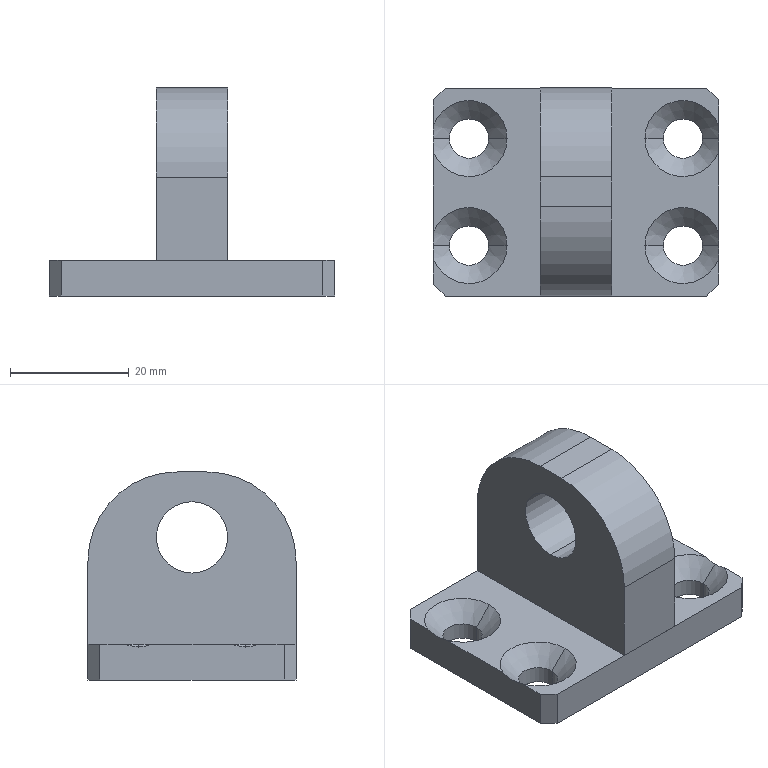Part | SolidWorks | features ICE 2, Chamfer 1, Extrusion 1, Fillet 1, HoleWzd 1 | 2 solids | 36 faces | box 48 x 35 x 35 mm | volume 18352 mm3 | plane 16 | cylinder 12 | cone 8 | commonest cylinder face diameters 6.6 x8 12 x2 30 x2
STEP:
#1=CARTESIAN_POINT('',(-6.,0.,30.));
#2=VERTEX_POINT('',#1);
#3=CARTESIAN_POINT('',(-6.,0.,18.));
#4=VERTEX_POINT('',#3);
#5=CARTESIAN_POINT('',(-6.,0.,24.));
#6=DIRECTION('',(1.,0.,0.));
#7=DIRECTION('',(0.,1.,0.));
#8=AXIS2_PLACEMENT_3D('',#5,#6,#7);
#9=CIRCLE('',#8,6.);
#10=EDGE_CURVE('',#2,#4,#9,.T.);
#11=ORIENTED_EDGE('',*,*,#10,.F.);
#12=CARTESIAN_POINT('',(6.,0.,30.));
#13=VERTEX_POINT('',#12);
#14=CARTESIAN_POINT('',(-14.,0.,30.));
#15=DIRECTION('',(1.,0.,0.));
#16=VECTOR('',#15,1000.);
#17=LINE('',#14,#16);
#18=EDGE_CURVE('',#2,#13,#17,.T.);
#19=ORIENTED_EDGE('',*,*,#18,.T.);
#20=CARTESIAN_POINT('',(6.,0.,18.));
#21=VERTEX_POINT('',#20);
#22=CARTESIAN_POINT('',(6.,0.,24.));
#23=DIRECTION('',(1.,0.,0.));
#24=DIRECTION('',(0.,0.,-1.));
#25=AXIS2_PLACEMENT_3D('',#22,#23,#24);
#26=CIRCLE('',#25,6.);
#27=EDGE_CURVE('',#13,#21,#26,.T.);
#28=ORIENTED_EDGE('',*,*,#27,.T.);
#29=CARTESIAN_POINT('',(-14.,0.,18.));
#30=DIRECTION('',(1.,0.,0.));
#31=VECTOR('',#30,1000.);
#32=LINE('',#29,#31);
#33=EDGE_CURVE('',#4,#21,#32,.T.);
#34=ORIENTED_EDGE('',*,*,#33,.F.);
#35=EDGE_LOOP('',(#11,#19,#28,#34));
#36=FACE_OUTER_BOUND('',#35,.T.);
#37=CARTESIAN_POINT('',(-14.,0.,24.));
#38=DIRECTION('',(1.,0.,0.));
#39=DIRECTION('',(0.,0.,-1.));
#40=AXIS2_PLACEMENT_3D('',#37,#38,#39);
#41=CYLINDRICAL_SURFACE('',#40,6.);
#42=ADVANCED_FACE('',(#36),#41,.F.);
#43=CARTESIAN_POINT('',(6.,0.,24.));
#44=DIRECTION('',(1.,0.,0.));
#45=DIRECTION('',(0.,0.,-1.));
#46=AXIS2_PLACEMENT_3D('',#43,#44,#45);
#47=CIRCLE('',#46,6.);
#48=EDGE_CURVE('',#21,#13,#47,.T.);
#49=ORIENTED_EDGE('',*,*,#48,.F.);
#50=ORIENTED_EDGE('',*,*,#27,.F.);
#51=EDGE_LOOP('',(#49,#50));
#52=FACE_BOUND('',#51,.T.);
#53=CARTESIAN_POINT('',(6.,-2.5,35.));
#54=VERTEX_POINT('',#53);
#55=CARTESIAN_POINT('',(6.,2.5,35.));
#56=VERTEX_POINT('',#55);
#57=CARTESIAN_POINT('',(6.,17.5,35.));
#58=DIRECTION('',(0.,1.,0.));
#59=VECTOR('',#58,1000.);
#60=LINE('',#57,#59);
#61=EDGE_CURVE('',#54,#56,#60,.T.);
#62=ORIENTED_EDGE('',*,*,#61,.F.);
#63=CARTESIAN_POINT('',(6.,-17.5,20.));
#64=VERTEX_POINT('',#63);
#65=CARTESIAN_POINT('',(6.,-2.5,20.));
#66=DIRECTION('',(1.,0.,0.));
#67=DIRECTION('',(0.,-1.,0.));
#68=AXIS2_PLACEMENT_3D('',#65,#66,#67);
#69=CIRCLE('',#68,15.);
#70=EDGE_CURVE('',#54,#64,#69,.T.);
#71=ORIENTED_EDGE('',*,*,#70,.T.);
#72=CARTESIAN_POINT('',(6.,-17.5,6.));
#73=VERTEX_POINT('',#72);
#74=CARTESIAN_POINT('',(6.,-17.5,35.));
#75=DIRECTION('',(0.,0.,-1.));
#76=VECTOR('',#75,1000.);
#77=LINE('',#74,#76);
#78=EDGE_CURVE('',#64,#73,#77,.T.);
#79=ORIENTED_EDGE('',*,*,#78,.T.);
#80=CARTESIAN_POINT('',(6.,17.5,6.));
#81=VERTEX_POINT('',#80);
#82=CARTESIAN_POINT('',(6.,17.5,6.));
#83=DIRECTION('',(0.,1.,0.));
#84=VECTOR('',#83,1000.);
#85=LINE('',#82,#84);
#86=EDGE_CURVE('',#73,#81,#85,.T.);
#87=ORIENTED_EDGE('',*,*,#86,.T.);
#88=CARTESIAN_POINT('',(6.,17.5,20.));
#89=VERTEX_POINT('',#88);
#90=CARTESIAN_POINT('',(6.,17.5,35.));
#91=DIRECTION('',(0.,0.,-1.));
#92=VECTOR('',#91,1000.);
#93=LINE('',#90,#92);
#94=EDGE_CURVE('',#89,#81,#93,.T.);
#95=ORIENTED_EDGE('',*,*,#94,.F.);
#96=CARTESIAN_POINT('',(6.,2.5,20.));
#97=DIRECTION('',(1.,0.,0.));
#98=DIRECTION('',(0.,-1.,0.));
#99=AXIS2_PLACEMENT_3D('',#96,#97,#98);
#100=CIRCLE('',#99,15.);
#101=EDGE_CURVE('',#89,#56,#100,.T.);
#102=ORIENTED_EDGE('',*,*,#101,.T.);
#103=EDGE_LOOP('',(#62,#71,#79,#87,#95,#102));
#104=FACE_OUTER_BOUND('',#103,.T.);
#105=CARTESIAN_POINT('',(6.,17.5,35.));
#106=DIRECTION('',(-1.,0.,0.));
#107=DIRECTION('',(0.,-1.,0.));
#108=AXIS2_PLACEMENT_3D('',#105,#106,#107);
#109=PLANE('',#108);
#110=ADVANCED_FACE('',(#52,#104),#109,.F.);
#111=CARTESIAN_POINT('',(-6.,17.5,20.));
#112=VERTEX_POINT('',#111);
#113=CARTESIAN_POINT('',(-6.,17.5,6.));
#114=VERTEX_POINT('',#113);
#115=CARTESIAN_POINT('',(-6.,17.5,35.));
#116=DIRECTION('',(0.,0.,-1.));
#117=VECTOR('',#116,1000.);
#118=LINE('',#115,#117);
#119=EDGE_CURVE('',#112,#114,#118,.T.);
#120=ORIENTED_EDGE('',*,*,#119,.F.);
#121=CARTESIAN_POINT('',(6.,17.5,20.));
#122=DIRECTION('',(1.,0.,0.));
#123=VECTOR('',#122,1000.);
#124=LINE('',#121,#123);
#125=EDGE_CURVE('',#112,#89,#124,.T.);
#126=ORIENTED_EDGE('',*,*,#125,.T.);
#127=ORIENTED_EDGE('',*,*,#94,.T.);
#128=CARTESIAN_POINT('',(-6.,17.5,6.));
#129=DIRECTION('',(-1.,0.,0.));
#130=VECTOR('',#129,1000.);
#131=LINE('',#128,#130);
#132=EDGE_CURVE('',#81,#114,#131,.T.);
#133=ORIENTED_EDGE('',*,*,#132,.T.);
#134=EDGE_LOOP('',(#120,#126,#127,#133));
#135=FACE_OUTER_BOUND('',#134,.T.);
#136=CARTESIAN_POINT('',(-6.,17.5,35.));
#137=DIRECTION('',(0.,-1.,0.));
#138=DIRECTION('',(0.,0.,-1.));
#139=AXIS2_PLACEMENT_3D('',#136,#137,#138);
#140=PLANE('',#139);
#141=ADVANCED_FACE('',(#135),#140,.F.);
#142=CARTESIAN_POINT('',(-6.,0.,24.));
#143=DIRECTION('',(1.,0.,0.));
#144=DIRECTION('',(0.,1.,0.));
#145=AXIS2_PLACEMENT_3D('',#142,#143,#144);
#146=CIRCLE('',#145,6.);
#147=EDGE_CURVE('',#4,#2,#146,.T.);
#148=ORIENTED_EDGE('',*,*,#147,.T.);
#149=ORIENTED_EDGE('',*,*,#10,.T.);
#150=EDGE_LOOP('',(#148,#149));
#151=FACE_BOUND('',#150,.T.);
#152=CARTESIAN_POINT('',(-6.,-17.5,20.));
#153=VERTEX_POINT('',#152);
#154=CARTESIAN_POINT('',(-6.,-17.5,6.));
#155=VERTEX_POINT('',#154);
#156=CARTESIAN_POINT('',(-6.,-17.5,35.));
#157=DIRECTION('',(0.,0.,-1.));
#158=VECTOR('',#157,1000.);
#159=LINE('',#156,#158);
#160=EDGE_CURVE('',#153,#155,#159,.T.);
#161=ORIENTED_EDGE('',*,*,#160,.F.);
#162=CARTESIAN_POINT('',(-6.,-2.5,35.));
#163=VERTEX_POINT('',#162);
#164=CARTESIAN_POINT('',(-6.,-2.5,20.));
#165=DIRECTION('',(-1.,0.,0.));
#166=DIRECTION('',(0.,1.,0.));
#167=AXIS2_PLACEMENT_3D('',#164,#165,#166);
#168=CIRCLE('',#167,15.);
#169=EDGE_CURVE('',#153,#163,#168,.T.);
#170=ORIENTED_EDGE('',*,*,#169,.T.);
#171=CARTESIAN_POINT('',(-6.,2.5,35.));
#172=VERTEX_POINT('',#171);
#173=CARTESIAN_POINT('',(-6.,17.5,35.));
#174=DIRECTION('',(0.,-1.,0.));
#175=VECTOR('',#174,1000.);
#176=LINE('',#173,#175);
#177=EDGE_CURVE('',#172,#163,#176,.T.);
#178=ORIENTED_EDGE('',*,*,#177,.F.);
#179=CARTESIAN_POINT('',(-6.,2.5,20.));
#180=DIRECTION('',(-1.,0.,0.));
#181=DIRECTION('',(0.,1.,0.));
#182=AXIS2_PLACEMENT_3D('',#179,#180,#181);
#183=CIRCLE('',#182,15.);
#184=EDGE_CURVE('',#172,#112,#183,.T.);
#185=ORIENTED_EDGE('',*,*,#184,.T.);
#186=ORIENTED_EDGE('',*,*,#119,.T.);
#187=CARTESIAN_POINT('',(-6.,17.5,6.));
#188=DIRECTION('',(0.,-1.,0.));
#189=VECTOR('',#188,1000.);
#190=LINE('',#187,#189);
#191=EDGE_CURVE('',#114,#155,#190,.T.);
#192=ORIENTED_EDGE('',*,*,#191,.T.);
#193=EDGE_LOOP('',(#161,#170,#178,#185,#186,#192));
#194=FACE_OUTER_BOUND('',#193,.T.);
#195=CARTESIAN_POINT('',(-6.,17.5,35.));
#196=DIRECTION('',(1.,0.,0.));
#197=DIRECTION('',(0.,1.,0.));
#198=AXIS2_PLACEMENT_3D('',#195,#196,#197);
#199=PLANE('',#198);
#200=ADVANCED_FACE('',(#151,#194),#199,.F.);
#201=ORIENTED_EDGE('',*,*,#78,.F.);
#202=CARTESIAN_POINT('',(-6.,-17.5,20.));
#203=DIRECTION('',(-1.,0.,0.));
#204=VECTOR('',#203,1000.);
#205=LINE('',#202,#204);
#206=EDGE_CURVE('',#64,#153,#205,.T.);
#207=ORIENTED_EDGE('',*,*,#206,.T.);
#208=ORIENTED_EDGE('',*,*,#160,.T.);
#209=CARTESIAN_POINT('',(-6.,-17.5,6.));
#210=DIRECTION('',(1.,0.,0.));
#211=VECTOR('',#210,1000.);
#212=LINE('',#209,#211);
#213=EDGE_CURVE('',#155,#73,#212,.T.);
#214=ORIENTED_EDGE('',*,*,#213,.T.);
#215=EDGE_LOOP('',(#201,#207,#208,#214));
#216=FACE_OUTER_BOUND('',#215,.T.);
#217=CARTESIAN_POINT('',(-6.,-17.5,35.));
#218=DIRECTION('',(0.,1.,0.));
#219=DIRECTION('',(0.,0.,1.));
#220=AXIS2_PLACEMENT_3D('',#217,#218,#219);
#221=PLANE('',#220);
#222=ADVANCED_FACE('',(#216),#221,.F.);
#223=ORIENTED_EDGE('',*,*,#177,.T.);
#224=CARTESIAN_POINT('',(6.,-2.5,35.));
#225=DIRECTION('',(1.,0.,0.));
#226=VECTOR('',#225,1000.);
#227=LINE('',#224,#226);
#228=EDGE_CURVE('',#163,#54,#227,.T.);
#229=ORIENTED_EDGE('',*,*,#228,.T.);
#230=ORIENTED_EDGE('',*,*,#61,.T.);
#231=CARTESIAN_POINT('',(-6.,2.5,35.));
#232=DIRECTION('',(-1.,0.,0.));
#233=VECTOR('',#232,1000.);
#234=LINE('',#231,#233);
#235=EDGE_CURVE('',#56,#172,#234,.T.);
#236=ORIENTED_EDGE('',*,*,#235,.T.);
#237=EDGE_LOOP('',(#223,#229,#230,#236));
#238=FACE_OUTER_BOUND('',#237,.T.);
#239=CARTESIAN_POINT('',(0.,0.,35.));
#240=DIRECTION('',(0.,0.,1.));
#241=DIRECTION('',(1.,0.,0.));
#242=AXIS2_PLACEMENT_3D('',#239,#240,#241);
#243=PLANE('',#242);
#244=ADVANCED_FACE('',(#238),#243,.T.);
#245=ORIENTED_EDGE('',*,*,#86,.F.);
#246=ORIENTED_EDGE('',*,*,#213,.F.);
#247=ORIENTED_EDGE('',*,*,#191,.F.);
#248=ORIENTED_EDGE('',*,*,#132,.F.);
#249=EDGE_LOOP('',(#245,#246,#247,#248));
#250=FACE_OUTER_BOUND('',#249,.T.);
#251=CARTESIAN_POINT('',(0.,0.,6.));
#252=DIRECTION('',(0.,0.,1.));
#253=DIRECTION('',(1.,0.,0.));
#254=AXIS2_PLACEMENT_3D('',#251,#252,#253);
#255=PLANE('',#254);
#256=ADVANCED_FACE('',(#250),#255,.F.);
#257=ORIENTED_EDGE('',*,*,#169,.F.);
#258=ORIENTED_EDGE('',*,*,#206,.F.);
#259=ORIENTED_EDGE('',*,*,#70,.F.);
#260=ORIENTED_EDGE('',*,*,#228,.F.);
#261=EDGE_LOOP('',(#257,#258,#259,#260));
#262=FACE_OUTER_BOUND('',#261,.T.);
#263=CARTESIAN_POINT('',(0.,-2.5,20.));
#264=DIRECTION('',(-1.,0.,0.));
#265=DIRECTION('',(0.,0.,1.));
#266=AXIS2_PLACEMENT_3D('',#263,#264,#265);
#267=CYLINDRICAL_SURFACE('',#266,15.);
#268=ADVANCED_FACE('',(#262),#267,.T.);
#269=ORIENTED_EDGE('',*,*,#101,.F.);
#270=ORIENTED_EDGE('',*,*,#125,.F.);
#271=ORIENTED_EDGE('',*,*,#184,.F.);
#272=ORIENTED_EDGE('',*,*,#235,.F.);
#273=EDGE_LOOP('',(#269,#270,#271,#272));
#274=FACE_OUTER_BOUND('',#273,.T.);
#275=CARTESIAN_POINT('',(0.,2.5,20.));
#276=DIRECTION('',(1.,0.,0.));
#277=DIRECTION('',(0.,0.,-1.));
#278=AXIS2_PLACEMENT_3D('',#275,#276,#277);
#279=CYLINDRICAL_SURFACE('',#278,15.);
#280=ADVANCED_FACE('',(#274),#279,.T.);
#281=ORIENTED_EDGE('',*,*,#18,.F.);
#282=ORIENTED_EDGE('',*,*,#147,.F.);
#283=ORIENTED_EDGE('',*,*,#33,.T.);
#284=ORIENTED_EDGE('',*,*,#48,.T.);
#285=EDGE_LOOP('',(#281,#282,#283,#284));
#286=FACE_OUTER_BOUND('',#285,.T.);
#287=CARTESIAN_POINT('',(-14.,0.,24.));
#288=DIRECTION('',(1.,0.,0.));
#289=DIRECTION('',(0.,0.,-1.));
#290=AXIS2_PLACEMENT_3D('',#287,#288,#289);
#291=CYLINDRICAL_SURFACE('',#290,6.);
#292=ADVANCED_FACE('',(#286),#291,.F.);
#293=CLOSED_SHELL('',(#42,#110,#141,#200,#222,#244,#256,#268,#280,#292));
#294=MANIFOLD_SOLID_BREP('',#293);
#295=CARTESIAN_POINT('',(-21.3,9.,0.));
#296=VERTEX_POINT('',#295);
#297=CARTESIAN_POINT('',(-14.7,9.,0.));
#298=VERTEX_POINT('',#297);
#299=CARTESIAN_POINT('',(-18.,9.,0.));
#300=DIRECTION('',(0.,0.,1.));
#301=DIRECTION('',(1.,0.,0.));
#302=AXIS2_PLACEMENT_3D('',#299,#300,#301);
#303=CIRCLE('',#302,3.3);
#304=EDGE_CURVE('',#296,#298,#303,.T.);
#305=ORIENTED_EDGE('',*,*,#304,.F.);
#306=CARTESIAN_POINT('',(-21.3,9.,2.9));
#307=VERTEX_POINT('',#306);
#308=CARTESIAN_POINT('',(-21.3,9.,6.));
#309=DIRECTION('',(0.,0.,1.));
#310=VECTOR('',#309,1000.);
#311=LINE('',#308,#310);
#312=EDGE_CURVE('',#296,#307,#311,.T.);
#313=ORIENTED_EDGE('',*,*,#312,.T.);
#314=CARTESIAN_POINT('',(-14.7,9.,2.9));
#315=VERTEX_POINT('',#314);
#316=CARTESIAN_POINT('',(-18.,9.,2.9));
#317=DIRECTION('',(0.,0.,1.));
#318=DIRECTION('',(1.,0.,0.));
#319=AXIS2_PLACEMENT_3D('',#316,#317,#318);
#320=CIRCLE('',#319,3.3);
#321=EDGE_CURVE('',#307,#315,#320,.T.);
#322=ORIENTED_EDGE('',*,*,#321,.T.);
#323=CARTESIAN_POINT('',(-14.7,9.,6.));
#324=DIRECTION('',(0.,0.,1.));
#325=VECTOR('',#324,1000.);
#326=LINE('',#323,#325);
#327=EDGE_CURVE('',#298,#315,#326,.T.);
#328=ORIENTED_EDGE('',*,*,#327,.F.);
#329=EDGE_LOOP('',(#305,#313,#322,#328));
#330=FACE_OUTER_BOUND('',#329,.T.);
#331=CARTESIAN_POINT('',(-18.,9.,6.));
#332=DIRECTION('',(0.,0.,1.));
#333=DIRECTION('',(1.,0.,0.));
#334=AXIS2_PLACEMENT_3D('',#331,#332,#333);
#335=CYLINDRICAL_SURFACE('',#334,3.3);
#336=ADVANCED_FACE('',(#330),#335,.F.);
#337=ORIENTED_EDGE('',*,*,#321,.F.);
#338=CARTESIAN_POINT('',(-24.,9.,5.6));
#339=VERTEX_POINT('',#338);
#340=CARTESIAN_POINT('',(-24.4,9.,6.));
#341=DIRECTION('',(-0.7071,0.,0.7071));
#342=VECTOR('',#341,1000.);
#343=LINE('',#340,#342);
#344=EDGE_CURVE('',#307,#339,#343,.T.);
#345=ORIENTED_EDGE('',*,*,#344,.T.);
#346=CARTESIAN_POINT('',(-24.,6.773,6.));
#347=VERTEX_POINT('',#346);
#348=CARTESIAN_POINT('',(-24.,6.773,6.));
#349=CARTESIAN_POINT('',(-24.,7.133,5.875));
#350=CARTESIAN_POINT('',(-24.,7.5,5.774));
#351=CARTESIAN_POINT('',(-24.,8.242,5.637));
#352=CARTESIAN_POINT('',(-24.,8.618,5.6));
#353=CARTESIAN_POINT('',(-24.,9.,5.6));
#354=B_SPLINE_CURVE_WITH_KNOTS('',3,(#348,#349,#350,#351,#352,#353),.UNSPECIFIED.,.F.,.F.,(4,2,4),(0.02504,0.02616,0.02729),.UNSPECIFIED.);
#355=EDGE_CURVE('',#347,#339,#354,.T.);
#356=ORIENTED_EDGE('',*,*,#355,.F.);
#357=CARTESIAN_POINT('',(-11.6,9.,6.));
#358=VERTEX_POINT('',#357);
#359=CARTESIAN_POINT('',(-18.,9.,6.));
#360=DIRECTION('',(0.,0.,1.));
#361=DIRECTION('',(1.,0.,0.));
#362=AXIS2_PLACEMENT_3D('',#359,#360,#361);
#363=CIRCLE('',#362,6.4);
#364=EDGE_CURVE('',#347,#358,#363,.T.);
#365=ORIENTED_EDGE('',*,*,#364,.T.);
#366=CARTESIAN_POINT('',(-11.6,9.,6.));
#367=DIRECTION('',(0.7071,0.,0.7071));
#368=VECTOR('',#367,1000.);
#369=LINE('',#366,#368);
#370=EDGE_CURVE('',#315,#358,#369,.T.);
#371=ORIENTED_EDGE('',*,*,#370,.F.);
#372=EDGE_LOOP('',(#337,#345,#356,#365,#371));
#373=FACE_OUTER_BOUND('',#372,.T.);
#374=CARTESIAN_POINT('',(-18.,9.,6.));
#375=DIRECTION('',(0.,0.,1.));
#376=DIRECTION('',(1.,0.,0.));
#377=AXIS2_PLACEMENT_3D('',#374,#375,#376);
#378=CONICAL_SURFACE('',#377,6.4,0.7854);
#379=ADVANCED_FACE('',(#373),#378,.F.);
#380=CARTESIAN_POINT('',(-21.3,-9.,0.));
#381=VERTEX_POINT('',#380);
#382=CARTESIAN_POINT('',(-14.7,-9.,0.));
#383=VERTEX_POINT('',#382);
#384=CARTESIAN_POINT('',(-18.,-9.,0.));
#385=DIRECTION('',(0.,0.,1.));
#386=DIRECTION('',(1.,0.,0.));
#387=AXIS2_PLACEMENT_3D('',#384,#385,#386);
#388=CIRCLE('',#387,3.3);
#389=EDGE_CURVE('',#381,#383,#388,.T.);
#390=ORIENTED_EDGE('',*,*,#389,.F.);
#391=CARTESIAN_POINT('',(-21.3,-9.,2.9));
#392=VERTEX_POINT('',#391);
#393=CARTESIAN_POINT('',(-21.3,-9.,6.));
#394=DIRECTION('',(0.,0.,1.));
#395=VECTOR('',#394,1000.);
#396=LINE('',#393,#395);
#397=EDGE_CURVE('',#381,#392,#396,.T.);
#398=ORIENTED_EDGE('',*,*,#397,.T.);
#399=CARTESIAN_POINT('',(-14.7,-9.,2.9));
#400=VERTEX_POINT('',#399);
#401=CARTESIAN_POINT('',(-18.,-9.,2.9));
#402=DIRECTION('',(0.,0.,1.));
#403=DIRECTION('',(1.,0.,0.));
#404=AXIS2_PLACEMENT_3D('',#401,#402,#403);
#405=CIRCLE('',#404,3.3);
#406=EDGE_CURVE('',#392,#400,#405,.T.);
#407=ORIENTED_EDGE('',*,*,#406,.T.);
#408=CARTESIAN_POINT('',(-14.7,-9.,6.));
#409=DIRECTION('',(0.,0.,1.));
#410=VECTOR('',#409,1000.);
#411=LINE('',#408,#410);
#412=EDGE_CURVE('',#383,#400,#411,.T.);
#413=ORIENTED_EDGE('',*,*,#412,.F.);
#414=EDGE_LOOP('',(#390,#398,#407,#413));
#415=FACE_OUTER_BOUND('',#414,.T.);
#416=CARTESIAN_POINT('',(-18.,-9.,6.));
#417=DIRECTION('',(0.,0.,1.));
#418=DIRECTION('',(1.,0.,0.));
#419=AXIS2_PLACEMENT_3D('',#416,#417,#418);
#420=CYLINDRICAL_SURFACE('',#419,3.3);
#421=ADVANCED_FACE('',(#415),#420,.F.);
#422=ORIENTED_EDGE('',*,*,#406,.F.);
#423=CARTESIAN_POINT('',(-24.,-9.,5.6));
#424=VERTEX_POINT('',#423);
#425=CARTESIAN_POINT('',(-24.4,-9.,6.));
#426=DIRECTION('',(-0.7071,0.,0.7071));
#427=VECTOR('',#426,1000.);
#428=LINE('',#425,#427);
#429=EDGE_CURVE('',#392,#424,#428,.T.);
#430=ORIENTED_EDGE('',*,*,#429,.T.);
#431=CARTESIAN_POINT('',(-24.,-11.227,6.));
#432=VERTEX_POINT('',#431);
#433=CARTESIAN_POINT('',(-24.,-11.227,6.));
#434=CARTESIAN_POINT('',(-24.,-10.867,5.875));
#435=CARTESIAN_POINT('',(-24.,-10.5,5.774));
#436=CARTESIAN_POINT('',(-24.,-9.758,5.637));
#437=CARTESIAN_POINT('',(-24.,-9.382,5.6));
#438=CARTESIAN_POINT('',(-24.,-9.,5.6));
#439=B_SPLINE_CURVE_WITH_KNOTS('',3,(#433,#434,#435,#436,#437,#438),.UNSPECIFIED.,.F.,.F.,(4,2,4),(0.02504,0.02616,0.02729),.UNSPECIFIED.);
#440=EDGE_CURVE('',#432,#424,#439,.T.);
#441=ORIENTED_EDGE('',*,*,#440,.F.);
#442=CARTESIAN_POINT('',(-11.6,-9.,6.));
#443=VERTEX_POINT('',#442);
#444=CARTESIAN_POINT('',(-18.,-9.,6.));
#445=DIRECTION('',(0.,0.,1.));
#446=DIRECTION('',(1.,0.,0.));
#447=AXIS2_PLACEMENT_3D('',#444,#445,#446);
#448=CIRCLE('',#447,6.4);
#449=EDGE_CURVE('',#432,#443,#448,.T.);
#450=ORIENTED_EDGE('',*,*,#449,.T.);
#451=CARTESIAN_POINT('',(-11.6,-9.,6.));
#452=DIRECTION('',(0.7071,0.,0.7071));
#453=VECTOR('',#452,1000.);
#454=LINE('',#451,#453);
#455=EDGE_CURVE('',#400,#443,#454,.T.);
#456=ORIENTED_EDGE('',*,*,#455,.F.);
#457=EDGE_LOOP('',(#422,#430,#441,#450,#456));
#458=FACE_OUTER_BOUND('',#457,.T.);
#459=CARTESIAN_POINT('',(-18.,-9.,6.));
#460=DIRECTION('',(0.,0.,1.));
#461=DIRECTION('',(1.,0.,0.));
#462=AXIS2_PLACEMENT_3D('',#459,#460,#461);
#463=CONICAL_SURFACE('',#462,6.4,0.7854);
#464=ADVANCED_FACE('',(#458),#463,.F.);
#465=CARTESIAN_POINT('',(14.7,9.,0.));
#466=VERTEX_POINT('',#465);
#467=CARTESIAN_POINT('',(21.3,9.,0.));
#468=VERTEX_POINT('',#467);
#469=CARTESIAN_POINT('',(18.,9.,0.));
#470=DIRECTION('',(0.,0.,1.));
#471=DIRECTION('',(1.,0.,0.));
#472=AXIS2_PLACEMENT_3D('',#469,#470,#471);
#473=CIRCLE('',#472,3.3);
#474=EDGE_CURVE('',#466,#468,#473,.T.);
#475=ORIENTED_EDGE('',*,*,#474,.F.);
#476=CARTESIAN_POINT('',(14.7,9.,2.9));
#477=VERTEX_POINT('',#476);
#478=CARTESIAN_POINT('',(14.7,9.,6.));
#479=DIRECTION('',(0.,0.,1.));
#480=VECTOR('',#479,1000.);
#481=LINE('',#478,#480);
#482=EDGE_CURVE('',#466,#477,#481,.T.);
#483=ORIENTED_EDGE('',*,*,#482,.T.);
#484=CARTESIAN_POINT('',(21.3,9.,2.9));
#485=VERTEX_POINT('',#484);
#486=CARTESIAN_POINT('',(18.,9.,2.9));
#487=DIRECTION('',(0.,0.,1.));
#488=DIRECTION('',(1.,0.,0.));
#489=AXIS2_PLACEMENT_3D('',#486,#487,#488);
#490=CIRCLE('',#489,3.3);
#491=EDGE_CURVE('',#477,#485,#490,.T.);
#492=ORIENTED_EDGE('',*,*,#491,.T.);
#493=CARTESIAN_POINT('',(21.3,9.,6.));
#494=DIRECTION('',(0.,0.,1.));
#495=VECTOR('',#494,1000.);
#496=LINE('',#493,#495);
#497=EDGE_CURVE('',#468,#485,#496,.T.);
#498=ORIENTED_EDGE('',*,*,#497,.F.);
#499=EDGE_LOOP('',(#475,#483,#492,#498));
#500=FACE_OUTER_BOUND('',#499,.T.);
#501=CARTESIAN_POINT('',(18.,9.,6.));
#502=DIRECTION('',(0.,0.,1.));
#503=DIRECTION('',(1.,0.,0.));
#504=AXIS2_PLACEMENT_3D('',#501,#502,#503);
#505=CYLINDRICAL_SURFACE('',#504,3.3);
#506=ADVANCED_FACE('',(#500),#505,.F.);
#507=ORIENTED_EDGE('',*,*,#491,.F.);
#508=CARTESIAN_POINT('',(11.6,9.,6.));
#509=VERTEX_POINT('',#508);
#510=CARTESIAN_POINT('',(11.6,9.,6.));
#511=DIRECTION('',(-0.7071,0.,0.7071));
#512=VECTOR('',#511,1000.);
#513=LINE('',#510,#512);
#514=EDGE_CURVE('',#477,#509,#513,.T.);
#515=ORIENTED_EDGE('',*,*,#514,.T.);
#516=CARTESIAN_POINT('',(24.,6.773,6.));
#517=VERTEX_POINT('',#516);
#518=CARTESIAN_POINT('',(18.,9.,6.));
#519=DIRECTION('',(0.,0.,1.));
#520=DIRECTION('',(1.,0.,0.));
#521=AXIS2_PLACEMENT_3D('',#518,#519,#520);
#522=CIRCLE('',#521,6.4);
#523=EDGE_CURVE('',#509,#517,#522,.T.);
#524=ORIENTED_EDGE('',*,*,#523,.T.);
#525=CARTESIAN_POINT('',(24.,9.,5.6));
#526=VERTEX_POINT('',#525);
#527=CARTESIAN_POINT('',(24.,9.,5.6));
#528=CARTESIAN_POINT('',(24.,8.618,5.6));
#529=CARTESIAN_POINT('',(24.,8.242,5.637));
#530=CARTESIAN_POINT('',(24.,7.5,5.774));
#531=CARTESIAN_POINT('',(24.,7.133,5.875));
#532=CARTESIAN_POINT('',(24.,6.773,6.));
#533=B_SPLINE_CURVE_WITH_KNOTS('',3,(#527,#528,#529,#530,#531,#532),.UNSPECIFIED.,.F.,.F.,(4,2,4),(0.03261,0.03374,0.03487),.UNSPECIFIED.);
#534=EDGE_CURVE('',#526,#517,#533,.T.);
#535=ORIENTED_EDGE('',*,*,#534,.F.);
#536=CARTESIAN_POINT('',(24.4,9.,6.));
#537=DIRECTION('',(0.7071,0.,0.7071));
#538=VECTOR('',#537,1000.);
#539=LINE('',#536,#538);
#540=EDGE_CURVE('',#485,#526,#539,.T.);
#541=ORIENTED_EDGE('',*,*,#540,.F.);
#542=EDGE_LOOP('',(#507,#515,#524,#535,#541));
#543=FACE_OUTER_BOUND('',#542,.T.);
#544=CARTESIAN_POINT('',(18.,9.,6.));
#545=DIRECTION('',(0.,0.,1.));
#546=DIRECTION('',(1.,0.,0.));
#547=AXIS2_PLACEMENT_3D('',#544,#545,#546);
#548=CONICAL_SURFACE('',#547,6.4,0.7854);
#549=ADVANCED_FACE('',(#543),#548,.F.);
#550=CARTESIAN_POINT('',(14.7,-9.,0.));
#551=VERTEX_POINT('',#550);
#552=CARTESIAN_POINT('',(21.3,-9.,0.));
#553=VERTEX_POINT('',#552);
#554=CARTESIAN_POINT('',(18.,-9.,0.));
#555=DIRECTION('',(0.,0.,1.));
#556=DIRECTION('',(1.,0.,0.));
#557=AXIS2_PLACEMENT_3D('',#554,#555,#556);
#558=CIRCLE('',#557,3.3);
#559=EDGE_CURVE('',#551,#553,#558,.T.);
#560=ORIENTED_EDGE('',*,*,#559,.F.);
#561=CARTESIAN_POINT('',(14.7,-9.,2.9));
#562=VERTEX_POINT('',#561);
#563=CARTESIAN_POINT('',(14.7,-9.,6.));
#564=DIRECTION('',(0.,0.,1.));
#565=VECTOR('',#564,1000.);
#566=LINE('',#563,#565);
#567=EDGE_CURVE('',#551,#562,#566,.T.);
#568=ORIENTED_EDGE('',*,*,#567,.T.);
#569=CARTESIAN_POINT('',(21.3,-9.,2.9));
#570=VERTEX_POINT('',#569);
#571=CARTESIAN_POINT('',(18.,-9.,2.9));
#572=DIRECTION('',(0.,0.,1.));
#573=DIRECTION('',(1.,0.,0.));
#574=AXIS2_PLACEMENT_3D('',#571,#572,#573);
#575=CIRCLE('',#574,3.3);
#576=EDGE_CURVE('',#562,#570,#575,.T.);
#577=ORIENTED_EDGE('',*,*,#576,.T.);
#578=CARTESIAN_POINT('',(21.3,-9.,6.));
#579=DIRECTION('',(0.,0.,1.));
#580=VECTOR('',#579,1000.);
#581=LINE('',#578,#580);
#582=EDGE_CURVE('',#553,#570,#581,.T.);
#583=ORIENTED_EDGE('',*,*,#582,.F.);
#584=EDGE_LOOP('',(#560,#568,#577,#583));
#585=FACE_OUTER_BOUND('',#584,.T.);
#586=CARTESIAN_POINT('',(18.,-9.,6.));
#587=DIRECTION('',(0.,0.,1.));
#588=DIRECTION('',(1.,0.,0.));
#589=AXIS2_PLACEMENT_3D('',#586,#587,#588);
#590=CYLINDRICAL_SURFACE('',#589,3.3);
#591=ADVANCED_FACE('',(#585),#590,.F.);
#592=ORIENTED_EDGE('',*,*,#576,.F.);
#593=CARTESIAN_POINT('',(11.6,-9.,6.));
#594=VERTEX_POINT('',#593);
#595=CARTESIAN_POINT('',(11.6,-9.,6.));
#596=DIRECTION('',(-0.7071,0.,0.7071));
#597=VECTOR('',#596,1000.);
#598=LINE('',#595,#597);
#599=EDGE_CURVE('',#562,#594,#598,.T.);
#600=ORIENTED_EDGE('',*,*,#599,.T.);
#601=CARTESIAN_POINT('',(24.,-11.227,6.));
#602=VERTEX_POINT('',#601);
#603=CARTESIAN_POINT('',(18.,-9.,6.));
#604=DIRECTION('',(0.,0.,1.));
#605=DIRECTION('',(1.,0.,0.));
#606=AXIS2_PLACEMENT_3D('',#603,#604,#605);
#607=CIRCLE('',#606,6.4);
#608=EDGE_CURVE('',#594,#602,#607,.T.);
#609=ORIENTED_EDGE('',*,*,#608,.T.);
#610=CARTESIAN_POINT('',(24.,-9.,5.6));
#611=VERTEX_POINT('',#610);
#612=CARTESIAN_POINT('',(24.,-9.,5.6));
#613=CARTESIAN_POINT('',(24.,-9.382,5.6));
#614=CARTESIAN_POINT('',(24.,-9.758,5.637));
#615=CARTESIAN_POINT('',(24.,-10.5,5.774));
#616=CARTESIAN_POINT('',(24.,-10.867,5.875));
#617=CARTESIAN_POINT('',(24.,-11.227,6.));
#618=B_SPLINE_CURVE_WITH_KNOTS('',3,(#612,#613,#614,#615,#616,#617),.UNSPECIFIED.,.F.,.F.,(4,2,4),(0.03261,0.03374,0.03487),.UNSPECIFIED.);
#619=EDGE_CURVE('',#611,#602,#618,.T.);
#620=ORIENTED_EDGE('',*,*,#619,.F.);
#621=CARTESIAN_POINT('',(24.4,-9.,6.));
#622=DIRECTION('',(0.7071,0.,0.7071));
#623=VECTOR('',#622,1000.);
#624=LINE('',#621,#623);
#625=EDGE_CURVE('',#570,#611,#624,.T.);
#626=ORIENTED_EDGE('',*,*,#625,.F.);
#627=EDGE_LOOP('',(#592,#600,#609,#620,#626));
#628=FACE_OUTER_BOUND('',#627,.T.);
#629=CARTESIAN_POINT('',(18.,-9.,6.));
#630=DIRECTION('',(0.,0.,1.));
#631=DIRECTION('',(1.,0.,0.));
#632=AXIS2_PLACEMENT_3D('',#629,#630,#631);
#633=CONICAL_SURFACE('',#632,6.4,0.7854);
#634=ADVANCED_FACE('',(#628),#633,.F.);
#635=CARTESIAN_POINT('',(24.,11.227,6.));
#636=VERTEX_POINT('',#635);
#637=CARTESIAN_POINT('',(24.,15.5,6.));
#638=VERTEX_POINT('',#637);
#639=CARTESIAN_POINT('',(24.,17.5,6.));
#640=DIRECTION('',(0.,1.,0.));
#641=VECTOR('',#640,1000.);
#642=LINE('',#639,#641);
#643=EDGE_CURVE('',#636,#638,#642,.T.);
#644=ORIENTED_EDGE('',*,*,#643,.F.);
#645=CARTESIAN_POINT('',(24.,11.227,6.));
#646=CARTESIAN_POINT('',(24.,10.868,5.875));
#647=CARTESIAN_POINT('',(24.,10.503,5.775));
#648=CARTESIAN_POINT('',(24.,9.947,5.671));
#649=CARTESIAN_POINT('',(24.,9.76,5.645));
#650=CARTESIAN_POINT('',(24.,9.382,5.609));
#651=CARTESIAN_POINT('',(24.,9.191,5.6));
#652=CARTESIAN_POINT('',(24.,9.,5.6));
#653=B_SPLINE_CURVE_WITH_KNOTS('',3,(#645,#646,#647,#648,#649,#650,#651,#652),.UNSPECIFIED.,.F.,.F.,(4,2,2,4),(0.03036,0.03149,0.03205,0.03261),.UNSPECIFIED.);
#654=EDGE_CURVE('',#636,#526,#653,.T.);
#655=ORIENTED_EDGE('',*,*,#654,.T.);
#656=ORIENTED_EDGE('',*,*,#534,.T.);
#657=CARTESIAN_POINT('',(24.,-6.773,6.));
#658=VERTEX_POINT('',#657);
#659=CARTESIAN_POINT('',(24.,17.5,6.));
#660=DIRECTION('',(0.,1.,0.));
#661=VECTOR('',#660,1000.);
#662=LINE('',#659,#661);
#663=EDGE_CURVE('',#658,#517,#662,.T.);
#664=ORIENTED_EDGE('',*,*,#663,.F.);
#665=CARTESIAN_POINT('',(24.,-6.773,6.));
#666=CARTESIAN_POINT('',(24.,-7.132,5.875));
#667=CARTESIAN_POINT('',(24.,-7.497,5.775));
#668=CARTESIAN_POINT('',(24.,-8.053,5.671));
#669=CARTESIAN_POINT('',(24.,-8.24,5.645));
#670=CARTESIAN_POINT('',(24.,-8.618,5.609));
#671=CARTESIAN_POINT('',(24.,-8.809,5.6));
#672=CARTESIAN_POINT('',(24.,-9.,5.6));
#673=B_SPLINE_CURVE_WITH_KNOTS('',3,(#665,#666,#667,#668,#669,#670,#671,#672),.UNSPECIFIED.,.F.,.F.,(4,2,2,4),(0.03036,0.03149,0.03205,0.03261),.UNSPECIFIED.);
#674=EDGE_CURVE('',#658,#611,#673,.T.);
#675=ORIENTED_EDGE('',*,*,#674,.T.);
#676=ORIENTED_EDGE('',*,*,#619,.T.);
#677=CARTESIAN_POINT('',(24.,-15.5,6.));
#678=VERTEX_POINT('',#677);
#679=CARTESIAN_POINT('',(24.,17.5,6.));
#680=DIRECTION('',(0.,1.,0.));
#681=VECTOR('',#680,1000.);
#682=LINE('',#679,#681);
#683=EDGE_CURVE('',#678,#602,#682,.T.);
#684=ORIENTED_EDGE('',*,*,#683,.F.);
#685=CARTESIAN_POINT('',(24.,-15.5,0.));
#686=VERTEX_POINT('',#685);
#687=CARTESIAN_POINT('',(24.,-15.5,6.));
#688=DIRECTION('',(0.,0.,-1.));
#689=VECTOR('',#688,1000.);
#690=LINE('',#687,#689);
#691=EDGE_CURVE('',#678,#686,#690,.T.);
#692=ORIENTED_EDGE('',*,*,#691,.T.);
#693=CARTESIAN_POINT('',(24.,15.5,0.));
#694=VERTEX_POINT('',#693);
#695=CARTESIAN_POINT('',(24.,17.5,0.));
#696=DIRECTION('',(0.,1.,0.));
#697=VECTOR('',#696,1000.);
#698=LINE('',#695,#697);
#699=EDGE_CURVE('',#686,#694,#698,.T.);
#700=ORIENTED_EDGE('',*,*,#699,.T.);
#701=CARTESIAN_POINT('',(24.,15.5,6.));
#702=DIRECTION('',(0.,0.,1.));
#703=VECTOR('',#702,1000.);
#704=LINE('',#701,#703);
#705=EDGE_CURVE('',#694,#638,#704,.T.);
#706=ORIENTED_EDGE('',*,*,#705,.T.);
#707=EDGE_LOOP('',(#644,#655,#656,#664,#675,#676,#684,#692,#700,#706));
#708=FACE_OUTER_BOUND('',#707,.T.);
#709=CARTESIAN_POINT('',(24.,17.5,6.));
#710=DIRECTION('',(-1.,0.,0.));
#711=DIRECTION('',(0.,-1.,0.));
#712=AXIS2_PLACEMENT_3D('',#709,#710,#711);
#713=PLANE('',#712);
#714=ADVANCED_FACE('',(#708),#713,.F.);
#715=CARTESIAN_POINT('',(22.,17.5,6.));
#716=VERTEX_POINT('',#715);
#717=CARTESIAN_POINT('',(-22.,17.5,6.));
#718=VERTEX_POINT('',#717);
#719=CARTESIAN_POINT('',(-24.,17.5,6.));
#720=DIRECTION('',(-1.,0.,0.));
#721=VECTOR('',#720,1000.);
#722=LINE('',#719,#721);
#723=EDGE_CURVE('',#716,#718,#722,.T.);
#724=ORIENTED_EDGE('',*,*,#723,.F.);
#725=CARTESIAN_POINT('',(22.,17.5,0.));
#726=VERTEX_POINT('',#725);
#727=CARTESIAN_POINT('',(22.,17.5,6.));
#728=DIRECTION('',(0.,0.,-1.));
#729=VECTOR('',#728,1000.);
#730=LINE('',#727,#729);
#731=EDGE_CURVE('',#716,#726,#730,.T.);
#732=ORIENTED_EDGE('',*,*,#731,.T.);
#733=CARTESIAN_POINT('',(-22.,17.5,0.));
#734=VERTEX_POINT('',#733);
#735=CARTESIAN_POINT('',(-24.,17.5,0.));
#736=DIRECTION('',(-1.,0.,0.));
#737=VECTOR('',#736,1000.);
#738=LINE('',#735,#737);
#739=EDGE_CURVE('',#726,#734,#738,.T.);
#740=ORIENTED_EDGE('',*,*,#739,.T.);
#741=CARTESIAN_POINT('',(-22.,17.5,6.));
#742=DIRECTION('',(0.,0.,1.));
#743=VECTOR('',#742,1000.);
#744=LINE('',#741,#743);
#745=EDGE_CURVE('',#734,#718,#744,.T.);
#746=ORIENTED_EDGE('',*,*,#745,.T.);
#747=EDGE_LOOP('',(#724,#732,#740,#746));
#748=FACE_OUTER_BOUND('',#747,.T.);
#749=CARTESIAN_POINT('',(-24.,17.5,6.));
#750=DIRECTION('',(0.,-1.,0.));
#751=DIRECTION('',(0.,0.,-1.));
#752=AXIS2_PLACEMENT_3D('',#749,#750,#751);
#753=PLANE('',#752);
#754=ADVANCED_FACE('',(#748),#753,.F.);
#755=CARTESIAN_POINT('',(-24.,-6.773,6.));
#756=VERTEX_POINT('',#755);
#757=CARTESIAN_POINT('',(-24.,17.5,6.));
#758=DIRECTION('',(0.,-1.,0.));
#759=VECTOR('',#758,1000.);
#760=LINE('',#757,#759);
#761=EDGE_CURVE('',#347,#756,#760,.T.);
#762=ORIENTED_EDGE('',*,*,#761,.F.);
#763=ORIENTED_EDGE('',*,*,#355,.T.);
#764=CARTESIAN_POINT('',(-24.,11.227,6.));
#765=VERTEX_POINT('',#764);
#766=CARTESIAN_POINT('',(-24.,9.,5.6));
#767=CARTESIAN_POINT('',(-24.,9.191,5.6));
#768=CARTESIAN_POINT('',(-24.,9.382,5.609));
#769=CARTESIAN_POINT('',(-24.,9.76,5.645));
#770=CARTESIAN_POINT('',(-24.,9.947,5.671));
#771=CARTESIAN_POINT('',(-24.,10.503,5.775));
#772=CARTESIAN_POINT('',(-24.,10.868,5.875));
#773=CARTESIAN_POINT('',(-24.,11.227,6.));
#774=B_SPLINE_CURVE_WITH_KNOTS('',3,(#766,#767,#768,#769,#770,#771,#772,#773),.UNSPECIFIED.,.F.,.F.,(4,2,2,4),(0.02729,0.02785,0.02841,0.02954),.UNSPECIFIED.);
#775=EDGE_CURVE('',#339,#765,#774,.T.);
#776=ORIENTED_EDGE('',*,*,#775,.T.);
#777=CARTESIAN_POINT('',(-24.,15.5,6.));
#778=VERTEX_POINT('',#777);
#779=CARTESIAN_POINT('',(-24.,17.5,6.));
#780=DIRECTION('',(0.,-1.,0.));
#781=VECTOR('',#780,1000.);
#782=LINE('',#779,#781);
#783=EDGE_CURVE('',#778,#765,#782,.T.);
#784=ORIENTED_EDGE('',*,*,#783,.F.);
#785=CARTESIAN_POINT('',(-24.,15.5,0.));
#786=VERTEX_POINT('',#785);
#787=CARTESIAN_POINT('',(-24.,15.5,6.));
#788=DIRECTION('',(0.,0.,-1.));
#789=VECTOR('',#788,1000.);
#790=LINE('',#787,#789);
#791=EDGE_CURVE('',#778,#786,#790,.T.);
#792=ORIENTED_EDGE('',*,*,#791,.T.);
#793=CARTESIAN_POINT('',(-24.,-15.5,0.));
#794=VERTEX_POINT('',#793);
#795=CARTESIAN_POINT('',(-24.,17.5,0.));
#796=DIRECTION('',(0.,-1.,0.));
#797=VECTOR('',#796,1000.);
#798=LINE('',#795,#797);
#799=EDGE_CURVE('',#786,#794,#798,.T.);
#800=ORIENTED_EDGE('',*,*,#799,.T.);
#801=CARTESIAN_POINT('',(-24.,-15.5,6.));
#802=VERTEX_POINT('',#801);
#803=CARTESIAN_POINT('',(-24.,-15.5,6.));
#804=DIRECTION('',(0.,0.,1.));
#805=VECTOR('',#804,1000.);
#806=LINE('',#803,#805);
#807=EDGE_CURVE('',#794,#802,#806,.T.);
#808=ORIENTED_EDGE('',*,*,#807,.T.);
#809=CARTESIAN_POINT('',(-24.,17.5,6.));
#810=DIRECTION('',(0.,-1.,0.));
#811=VECTOR('',#810,1000.);
#812=LINE('',#809,#811);
#813=EDGE_CURVE('',#432,#802,#812,.T.);
#814=ORIENTED_EDGE('',*,*,#813,.F.);
#815=ORIENTED_EDGE('',*,*,#440,.T.);
#816=CARTESIAN_POINT('',(-24.,-9.,5.6));
#817=CARTESIAN_POINT('',(-24.,-8.809,5.6));
#818=CARTESIAN_POINT('',(-24.,-8.618,5.609));
#819=CARTESIAN_POINT('',(-24.,-8.24,5.645));
#820=CARTESIAN_POINT('',(-24.,-8.053,5.671));
#821=CARTESIAN_POINT('',(-24.,-7.497,5.775));
#822=CARTESIAN_POINT('',(-24.,-7.132,5.875));
#823=CARTESIAN_POINT('',(-24.,-6.773,6.));
#824=B_SPLINE_CURVE_WITH_KNOTS('',3,(#816,#817,#818,#819,#820,#821,#822,#823),.UNSPECIFIED.,.F.,.F.,(4,2,2,4),(0.02729,0.02785,0.02841,0.02954),.UNSPECIFIED.);
#825=EDGE_CURVE('',#424,#756,#824,.T.);
#826=ORIENTED_EDGE('',*,*,#825,.T.);
#827=EDGE_LOOP('',(#762,#763,#776,#784,#792,#800,#808,#814,#815,#826));
#828=FACE_OUTER_BOUND('',#827,.T.);
#829=CARTESIAN_POINT('',(-24.,17.5,6.));
#830=DIRECTION('',(1.,0.,0.));
#831=DIRECTION('',(0.,1.,0.));
#832=AXIS2_PLACEMENT_3D('',#829,#830,#831);
#833=PLANE('',#832);
#834=ADVANCED_FACE('',(#828),#833,.F.);
#835=CARTESIAN_POINT('',(-22.,-17.5,0.));
#836=VERTEX_POINT('',#835);
#837=CARTESIAN_POINT('',(22.,-17.5,0.));
#838=VERTEX_POINT('',#837);
#839=CARTESIAN_POINT('',(-24.,-17.5,0.));
#840=DIRECTION('',(1.,0.,0.));
#841=VECTOR('',#840,1000.);
#842=LINE('',#839,#841);
#843=EDGE_CURVE('',#836,#838,#842,.T.);
#844=ORIENTED_EDGE('',*,*,#843,.T.);
#845=CARTESIAN_POINT('',(22.,-17.5,6.));
#846=VERTEX_POINT('',#845);
#847=CARTESIAN_POINT('',(22.,-17.5,6.));
#848=DIRECTION('',(0.,0.,1.));
#849=VECTOR('',#848,1000.);
#850=LINE('',#847,#849);
#851=EDGE_CURVE('',#838,#846,#850,.T.);
#852=ORIENTED_EDGE('',*,*,#851,.T.);
#853=CARTESIAN_POINT('',(-22.,-17.5,6.));
#854=VERTEX_POINT('',#853);
#855=CARTESIAN_POINT('',(-24.,-17.5,6.));
#856=DIRECTION('',(1.,0.,0.));
#857=VECTOR('',#856,1000.);
#858=LINE('',#855,#857);
#859=EDGE_CURVE('',#854,#846,#858,.T.);
#860=ORIENTED_EDGE('',*,*,#859,.F.);
#861=CARTESIAN_POINT('',(-22.,-17.5,6.));
#862=DIRECTION('',(0.,0.,-1.));
#863=VECTOR('',#862,1000.);
#864=LINE('',#861,#863);
#865=EDGE_CURVE('',#854,#836,#864,.T.);
#866=ORIENTED_EDGE('',*,*,#865,.T.);
#867=EDGE_LOOP('',(#844,#852,#860,#866));
#868=FACE_OUTER_BOUND('',#867,.T.);
#869=CARTESIAN_POINT('',(-24.,-17.5,6.));
#870=DIRECTION('',(0.,1.,0.));
#871=DIRECTION('',(0.,0.,1.));
#872=AXIS2_PLACEMENT_3D('',#869,#870,#871);
#873=PLANE('',#872);
#874=ADVANCED_FACE('',(#868),#873,.F.);
#875=ORIENTED_EDGE('',*,*,#364,.F.);
#876=ORIENTED_EDGE('',*,*,#761,.T.);
#877=CARTESIAN_POINT('',(-18.,-9.,6.));
#878=DIRECTION('',(0.,0.,1.));
#879=DIRECTION('',(1.,0.,0.));
#880=AXIS2_PLACEMENT_3D('',#877,#878,#879);
#881=CIRCLE('',#880,6.4);
#882=EDGE_CURVE('',#443,#756,#881,.T.);
#883=ORIENTED_EDGE('',*,*,#882,.F.);
#884=ORIENTED_EDGE('',*,*,#449,.F.);
#885=ORIENTED_EDGE('',*,*,#813,.T.);
#886=CARTESIAN_POINT('',(-19.75,-19.75,6.));
#887=DIRECTION('',(0.7071,-0.7071,0.));
#888=VECTOR('',#887,1000.);
#889=LINE('',#886,#888);
#890=EDGE_CURVE('',#802,#854,#889,.T.);
#891=ORIENTED_EDGE('',*,*,#890,.T.);
#892=ORIENTED_EDGE('',*,*,#859,.T.);
#893=CARTESIAN_POINT('',(19.75,-19.75,6.));
#894=DIRECTION('',(0.7071,0.7071,0.));
#895=VECTOR('',#894,1000.);
#896=LINE('',#893,#895);
#897=EDGE_CURVE('',#846,#678,#896,.T.);
#898=ORIENTED_EDGE('',*,*,#897,.T.);
#899=ORIENTED_EDGE('',*,*,#683,.T.);
#900=ORIENTED_EDGE('',*,*,#608,.F.);
#901=CARTESIAN_POINT('',(18.,-9.,6.));
#902=DIRECTION('',(0.,0.,1.));
#903=DIRECTION('',(1.,0.,0.));
#904=AXIS2_PLACEMENT_3D('',#901,#902,#903);
#905=CIRCLE('',#904,6.4);
#906=EDGE_CURVE('',#658,#594,#905,.T.);
#907=ORIENTED_EDGE('',*,*,#906,.F.);
#908=ORIENTED_EDGE('',*,*,#663,.T.);
#909=ORIENTED_EDGE('',*,*,#523,.F.);
#910=CARTESIAN_POINT('',(18.,9.,6.));
#911=DIRECTION('',(0.,0.,1.));
#912=DIRECTION('',(1.,0.,0.));
#913=AXIS2_PLACEMENT_3D('',#910,#911,#912);
#914=CIRCLE('',#913,6.4);
#915=EDGE_CURVE('',#636,#509,#914,.T.);
#916=ORIENTED_EDGE('',*,*,#915,.F.);
#917=ORIENTED_EDGE('',*,*,#643,.T.);
#918=CARTESIAN_POINT('',(19.75,19.75,6.));
#919=DIRECTION('',(-0.7071,0.7071,0.));
#920=VECTOR('',#919,1000.);
#921=LINE('',#918,#920);
#922=EDGE_CURVE('',#638,#716,#921,.T.);
#923=ORIENTED_EDGE('',*,*,#922,.T.);
#924=ORIENTED_EDGE('',*,*,#723,.T.);
#925=CARTESIAN_POINT('',(-19.75,19.75,6.));
#926=DIRECTION('',(-0.7071,-0.7071,0.));
#927=VECTOR('',#926,1000.);
#928=LINE('',#925,#927);
#929=EDGE_CURVE('',#718,#778,#928,.T.);
#930=ORIENTED_EDGE('',*,*,#929,.T.);
#931=ORIENTED_EDGE('',*,*,#783,.T.);
#932=CARTESIAN_POINT('',(-18.,9.,6.));
#933=DIRECTION('',(0.,0.,1.));
#934=DIRECTION('',(1.,0.,0.));
#935=AXIS2_PLACEMENT_3D('',#932,#933,#934);
#936=CIRCLE('',#935,6.4);
#937=EDGE_CURVE('',#358,#765,#936,.T.);
#938=ORIENTED_EDGE('',*,*,#937,.F.);
#939=EDGE_LOOP('',(#875,#876,#883,#884,#885,#891,#892,#898,#899,#900,#907,#908,#909,#916,#917,#923,#924,#930,#931,#938));
#940=FACE_OUTER_BOUND('',#939,.T.);
#941=CARTESIAN_POINT('',(0.,0.,6.));
#942=DIRECTION('',(0.,0.,1.));
#943=DIRECTION('',(1.,0.,0.));
#944=AXIS2_PLACEMENT_3D('',#941,#942,#943);
#945=PLANE('',#944);
#946=ADVANCED_FACE('',(#940),#945,.T.);
#947=CARTESIAN_POINT('',(-18.,9.,0.));
#948=DIRECTION('',(0.,0.,1.));
#949=DIRECTION('',(1.,0.,0.));
#950=AXIS2_PLACEMENT_3D('',#947,#948,#949);
#951=CIRCLE('',#950,3.3);
#952=EDGE_CURVE('',#298,#296,#951,.T.);
#953=ORIENTED_EDGE('',*,*,#952,.T.);
#954=ORIENTED_EDGE('',*,*,#304,.T.);
#955=EDGE_LOOP('',(#953,#954));
#956=FACE_BOUND('',#955,.T.);
#957=CARTESIAN_POINT('',(-18.,-9.,0.));
#958=DIRECTION('',(0.,0.,1.));
#959=DIRECTION('',(1.,0.,0.));
#960=AXIS2_PLACEMENT_3D('',#957,#958,#959);
#961=CIRCLE('',#960,3.3);
#962=EDGE_CURVE('',#383,#381,#961,.T.);
#963=ORIENTED_EDGE('',*,*,#962,.T.);
#964=ORIENTED_EDGE('',*,*,#389,.T.);
#965=EDGE_LOOP('',(#963,#964));
#966=FACE_BOUND('',#965,.T.);
#967=CARTESIAN_POINT('',(18.,9.,0.));
#968=DIRECTION('',(0.,0.,1.));
#969=DIRECTION('',(1.,0.,0.));
#970=AXIS2_PLACEMENT_3D('',#967,#968,#969);
#971=CIRCLE('',#970,3.3);
#972=EDGE_CURVE('',#468,#466,#971,.T.);
#973=ORIENTED_EDGE('',*,*,#972,.T.);
#974=ORIENTED_EDGE('',*,*,#474,.T.);
#975=EDGE_LOOP('',(#973,#974));
#976=FACE_BOUND('',#975,.T.);
#977=CARTESIAN_POINT('',(18.,-9.,0.));
#978=DIRECTION('',(0.,0.,1.));
#979=DIRECTION('',(1.,0.,0.));
#980=AXIS2_PLACEMENT_3D('',#977,#978,#979);
#981=CIRCLE('',#980,3.3);
#982=EDGE_CURVE('',#553,#551,#981,.T.);
#983=ORIENTED_EDGE('',*,*,#982,.T.);
#984=ORIENTED_EDGE('',*,*,#559,.T.);
#985=EDGE_LOOP('',(#983,#984));
#986=FACE_BOUND('',#985,.T.);
#987=ORIENTED_EDGE('',*,*,#739,.F.);
#988=CARTESIAN_POINT('',(22.,17.5,0.));
#989=DIRECTION('',(0.7071,-0.7071,0.));
#990=VECTOR('',#989,1000.);
#991=LINE('',#988,#990);
#992=EDGE_CURVE('',#726,#694,#991,.T.);
#993=ORIENTED_EDGE('',*,*,#992,.T.);
#994=ORIENTED_EDGE('',*,*,#699,.F.);
#995=CARTESIAN_POINT('',(24.,-15.5,0.));
#996=DIRECTION('',(-0.7071,-0.7071,0.));
#997=VECTOR('',#996,1000.);
#998=LINE('',#995,#997);
#999=EDGE_CURVE('',#686,#838,#998,.T.);
#1000=ORIENTED_EDGE('',*,*,#999,.T.);
#1001=ORIENTED_EDGE('',*,*,#843,.F.);
#1002=CARTESIAN_POINT('',(-22.,-17.5,0.));
#1003=DIRECTION('',(-0.7071,0.7071,0.));
#1004=VECTOR('',#1003,1000.);
#1005=LINE('',#1002,#1004);
#1006=EDGE_CURVE('',#836,#794,#1005,.T.);
#1007=ORIENTED_EDGE('',*,*,#1006,.T.);
#1008=ORIENTED_EDGE('',*,*,#799,.F.);
#1009=CARTESIAN_POINT('',(-24.,15.5,0.));
#1010=DIRECTION('',(0.7071,0.7071,0.));
#1011=VECTOR('',#1010,1000.);
#1012=LINE('',#1009,#1011);
#1013=EDGE_CURVE('',#786,#734,#1012,.T.);
#1014=ORIENTED_EDGE('',*,*,#1013,.T.);
#1015=EDGE_LOOP('',(#987,#993,#994,#1000,#1001,#1007,#1008,#1014));
#1016=FACE_OUTER_BOUND('',#1015,.T.);
#1017=CARTESIAN_POINT('',(0.,0.,0.));
#1018=DIRECTION('',(0.,0.,1.));
#1019=DIRECTION('',(1.,0.,0.));
#1020=AXIS2_PLACEMENT_3D('',#1017,#1018,#1019);
#1021=PLANE('',#1020);
#1022=ADVANCED_FACE('',(#956,#966,#976,#986,#1016),#1021,.F.);
#1023=ORIENTED_EDGE('',*,*,#922,.F.);
#1024=ORIENTED_EDGE('',*,*,#705,.F.);
#1025=ORIENTED_EDGE('',*,*,#992,.F.);
#1026=ORIENTED_EDGE('',*,*,#731,.F.);
#1027=EDGE_LOOP('',(#1023,#1024,#1025,#1026));
#1028=FACE_OUTER_BOUND('',#1027,.T.);
#1029=CARTESIAN_POINT('',(22.,17.5,6.));
#1030=DIRECTION('',(-0.7071,-0.7071,0.));
#1031=DIRECTION('',(0.,0.,-1.));
#1032=AXIS2_PLACEMENT_3D('',#1029,#1030,#1031);
#1033=PLANE('',#1032);
#1034=ADVANCED_FACE('',(#1028),#1033,.F.);
#1035=ORIENTED_EDGE('',*,*,#897,.F.);
#1036=ORIENTED_EDGE('',*,*,#851,.F.);
#1037=ORIENTED_EDGE('',*,*,#999,.F.);
#1038=ORIENTED_EDGE('',*,*,#691,.F.);
#1039=EDGE_LOOP('',(#1035,#1036,#1037,#1038));
#1040=FACE_OUTER_BOUND('',#1039,.T.);
#1041=CARTESIAN_POINT('',(24.,-15.5,6.));
#1042=DIRECTION('',(-0.7071,0.7071,0.));
#1043=DIRECTION('',(0.,0.,-1.));
#1044=AXIS2_PLACEMENT_3D('',#1041,#1042,#1043);
#1045=PLANE('',#1044);
#1046=ADVANCED_FACE('',(#1040),#1045,.F.);
#1047=ORIENTED_EDGE('',*,*,#890,.F.);
#1048=ORIENTED_EDGE('',*,*,#807,.F.);
#1049=ORIENTED_EDGE('',*,*,#1006,.F.);
#1050=ORIENTED_EDGE('',*,*,#865,.F.);
#1051=EDGE_LOOP('',(#1047,#1048,#1049,#1050));
#1052=FACE_OUTER_BOUND('',#1051,.T.);
#1053=CARTESIAN_POINT('',(-22.,-17.5,6.));
#1054=DIRECTION('',(0.7071,0.7071,0.));
#1055=DIRECTION('',(0.,0.,-1.));
#1056=AXIS2_PLACEMENT_3D('',#1053,#1054,#1055);
#1057=PLANE('',#1056);
#1058=ADVANCED_FACE('',(#1052),#1057,.F.);
#1059=ORIENTED_EDGE('',*,*,#929,.F.);
#1060=ORIENTED_EDGE('',*,*,#745,.F.);
#1061=ORIENTED_EDGE('',*,*,#1013,.F.);
#1062=ORIENTED_EDGE('',*,*,#791,.F.);
#1063=EDGE_LOOP('',(#1059,#1060,#1061,#1062));
#1064=FACE_OUTER_BOUND('',#1063,.T.);
#1065=CARTESIAN_POINT('',(-24.,15.5,6.));
#1066=DIRECTION('',(0.7071,-0.7071,0.));
#1067=DIRECTION('',(0.,0.,-1.));
#1068=AXIS2_PLACEMENT_3D('',#1065,#1066,#1067);
#1069=PLANE('',#1068);
#1070=ADVANCED_FACE('',(#1064),#1069,.F.);
#1071=ORIENTED_EDGE('',*,*,#599,.F.);
#1072=CARTESIAN_POINT('',(18.,-9.,2.9));
#1073=DIRECTION('',(0.,0.,1.));
#1074=DIRECTION('',(1.,0.,0.));
#1075=AXIS2_PLACEMENT_3D('',#1072,#1073,#1074);
#1076=CIRCLE('',#1075,3.3);
#1077=EDGE_CURVE('',#570,#562,#1076,.T.);
#1078=ORIENTED_EDGE('',*,*,#1077,.F.);
#1079=ORIENTED_EDGE('',*,*,#625,.T.);
#1080=ORIENTED_EDGE('',*,*,#674,.F.);
#1081=ORIENTED_EDGE('',*,*,#906,.T.);
#1082=EDGE_LOOP('',(#1071,#1078,#1079,#1080,#1081));
#1083=FACE_OUTER_BOUND('',#1082,.T.);
#1084=CARTESIAN_POINT('',(18.,-9.,6.));
#1085=DIRECTION('',(0.,0.,1.));
#1086=DIRECTION('',(1.,0.,0.));
#1087=AXIS2_PLACEMENT_3D('',#1084,#1085,#1086);
#1088=CONICAL_SURFACE('',#1087,6.4,0.7854);
#1089=ADVANCED_FACE('',(#1083),#1088,.F.);
#1090=ORIENTED_EDGE('',*,*,#567,.F.);
#1091=ORIENTED_EDGE('',*,*,#982,.F.);
#1092=ORIENTED_EDGE('',*,*,#582,.T.);
#1093=ORIENTED_EDGE('',*,*,#1077,.T.);
#1094=EDGE_LOOP('',(#1090,#1091,#1092,#1093));
#1095=FACE_OUTER_BOUND('',#1094,.T.);
#1096=CARTESIAN_POINT('',(18.,-9.,6.));
#1097=DIRECTION('',(0.,0.,1.));
#1098=DIRECTION('',(1.,0.,0.));
#1099=AXIS2_PLACEMENT_3D('',#1096,#1097,#1098);
#1100=CYLINDRICAL_SURFACE('',#1099,3.3);
#1101=ADVANCED_FACE('',(#1095),#1100,.F.);
#1102=ORIENTED_EDGE('',*,*,#514,.F.);
#1103=CARTESIAN_POINT('',(18.,9.,2.9));
#1104=DIRECTION('',(0.,0.,1.));
#1105=DIRECTION('',(1.,0.,0.));
#1106=AXIS2_PLACEMENT_3D('',#1103,#1104,#1105);
#1107=CIRCLE('',#1106,3.3);
#1108=EDGE_CURVE('',#485,#477,#1107,.T.);
#1109=ORIENTED_EDGE('',*,*,#1108,.F.);
#1110=ORIENTED_EDGE('',*,*,#540,.T.);
#1111=ORIENTED_EDGE('',*,*,#654,.F.);
#1112=ORIENTED_EDGE('',*,*,#915,.T.);
#1113=EDGE_LOOP('',(#1102,#1109,#1110,#1111,#1112));
#1114=FACE_OUTER_BOUND('',#1113,.T.);
#1115=CARTESIAN_POINT('',(18.,9.,6.));
#1116=DIRECTION('',(0.,0.,1.));
#1117=DIRECTION('',(1.,0.,0.));
#1118=AXIS2_PLACEMENT_3D('',#1115,#1116,#1117);
#1119=CONICAL_SURFACE('',#1118,6.4,0.7854);
#1120=ADVANCED_FACE('',(#1114),#1119,.F.);
#1121=ORIENTED_EDGE('',*,*,#482,.F.);
#1122=ORIENTED_EDGE('',*,*,#972,.F.);
#1123=ORIENTED_EDGE('',*,*,#497,.T.);
#1124=ORIENTED_EDGE('',*,*,#1108,.T.);
#1125=EDGE_LOOP('',(#1121,#1122,#1123,#1124));
#1126=FACE_OUTER_BOUND('',#1125,.T.);
#1127=CARTESIAN_POINT('',(18.,9.,6.));
#1128=DIRECTION('',(0.,0.,1.));
#1129=DIRECTION('',(1.,0.,0.));
#1130=AXIS2_PLACEMENT_3D('',#1127,#1128,#1129);
#1131=CYLINDRICAL_SURFACE('',#1130,3.3);
#1132=ADVANCED_FACE('',(#1126),#1131,.F.);
#1133=ORIENTED_EDGE('',*,*,#429,.F.);
#1134=CARTESIAN_POINT('',(-18.,-9.,2.9));
#1135=DIRECTION('',(0.,0.,1.));
#1136=DIRECTION('',(1.,0.,0.));
#1137=AXIS2_PLACEMENT_3D('',#1134,#1135,#1136);
#1138=CIRCLE('',#1137,3.3);
#1139=EDGE_CURVE('',#400,#392,#1138,.T.);
#1140=ORIENTED_EDGE('',*,*,#1139,.F.);
#1141=ORIENTED_EDGE('',*,*,#455,.T.);
#1142=ORIENTED_EDGE('',*,*,#882,.T.);
#1143=ORIENTED_EDGE('',*,*,#825,.F.);
#1144=EDGE_LOOP('',(#1133,#1140,#1141,#1142,#1143));
#1145=FACE_OUTER_BOUND('',#1144,.T.);
#1146=CARTESIAN_POINT('',(-18.,-9.,6.));
#1147=DIRECTION('',(0.,0.,1.));
#1148=DIRECTION('',(1.,0.,0.));
#1149=AXIS2_PLACEMENT_3D('',#1146,#1147,#1148);
#1150=CONICAL_SURFACE('',#1149,6.4,0.7854);
#1151=ADVANCED_FACE('',(#1145),#1150,.F.);
#1152=ORIENTED_EDGE('',*,*,#397,.F.);
#1153=ORIENTED_EDGE('',*,*,#962,.F.);
#1154=ORIENTED_EDGE('',*,*,#412,.T.);
#1155=ORIENTED_EDGE('',*,*,#1139,.T.);
#1156=EDGE_LOOP('',(#1152,#1153,#1154,#1155));
#1157=FACE_OUTER_BOUND('',#1156,.T.);
#1158=CARTESIAN_POINT('',(-18.,-9.,6.));
#1159=DIRECTION('',(0.,0.,1.));
#1160=DIRECTION('',(1.,0.,0.));
#1161=AXIS2_PLACEMENT_3D('',#1158,#1159,#1160);
#1162=CYLINDRICAL_SURFACE('',#1161,3.3);
#1163=ADVANCED_FACE('',(#1157),#1162,.F.);
#1164=ORIENTED_EDGE('',*,*,#344,.F.);
#1165=CARTESIAN_POINT('',(-18.,9.,2.9));
#1166=DIRECTION('',(0.,0.,1.));
#1167=DIRECTION('',(1.,0.,0.));
#1168=AXIS2_PLACEMENT_3D('',#1165,#1166,#1167);
#1169=CIRCLE('',#1168,3.3);
#1170=EDGE_CURVE('',#315,#307,#1169,.T.);
#1171=ORIENTED_EDGE('',*,*,#1170,.F.);
#1172=ORIENTED_EDGE('',*,*,#370,.T.);
#1173=ORIENTED_EDGE('',*,*,#937,.T.);
#1174=ORIENTED_EDGE('',*,*,#775,.F.);
#1175=EDGE_LOOP('',(#1164,#1171,#1172,#1173,#1174));
#1176=FACE_OUTER_BOUND('',#1175,.T.);
#1177=CARTESIAN_POINT('',(-18.,9.,6.));
#1178=DIRECTION('',(0.,0.,1.));
#1179=DIRECTION('',(1.,0.,0.));
#1180=AXIS2_PLACEMENT_3D('',#1177,#1178,#1179);
#1181=CONICAL_SURFACE('',#1180,6.4,0.7854);
#1182=ADVANCED_FACE('',(#1176),#1181,.F.);
#1183=ORIENTED_EDGE('',*,*,#312,.F.);
#1184=ORIENTED_EDGE('',*,*,#952,.F.);
#1185=ORIENTED_EDGE('',*,*,#327,.T.);
#1186=ORIENTED_EDGE('',*,*,#1170,.T.);
#1187=EDGE_LOOP('',(#1183,#1184,#1185,#1186));
#1188=FACE_OUTER_BOUND('',#1187,.T.);
#1189=CARTESIAN_POINT('',(-18.,9.,6.));
#1190=DIRECTION('',(0.,0.,1.));
#1191=DIRECTION('',(1.,0.,0.));
#1192=AXIS2_PLACEMENT_3D('',#1189,#1190,#1191);
#1193=CYLINDRICAL_SURFACE('',#1192,3.3);
#1194=ADVANCED_FACE('',(#1188),#1193,.F.);
#1195=CLOSED_SHELL('',(#336,#379,#421,#464,#506,#549,#591,#634,#714,#754,#834,#874,#946,#1022,#1034,#1046,#1058,#1070,#1089,#1101,#1120,#1132,#1151,#1163,#1182,#1194));
#1196=MANIFOLD_SOLID_BREP('',#1195);
#1197=CARTESIAN_POINT('',(0.,0.,0.));
#1198=DIRECTION('',(0.,0.,1.));
#1199=DIRECTION('',(1.,0.,0.));
#1200=AXIS2_PLACEMENT_3D('',#1197,#1198,#1199);
#1201=(LENGTH_UNIT()NAMED_UNIT(*)SI_UNIT(.MILLI.,.METRE.));
#1202=UNCERTAINTY_MEASURE_WITH_UNIT(LENGTH_MEASURE(0.00001),#1201,'','');
#1203=(NAMED_UNIT(*)PLANE_ANGLE_UNIT()SI_UNIT($,.RADIAN.));
#1204=(NAMED_UNIT(*)SI_UNIT($,.STERADIAN.)SOLID_ANGLE_UNIT());
#1205=(GEOMETRIC_REPRESENTATION_CONTEXT(3)GLOBAL_UNCERTAINTY_ASSIGNED_CONTEXT((#1202))GLOBAL_UNIT_ASSIGNED_CONTEXT((#1201,#1203,#1204))REPRESENTATION_CONTEXT('',''));
#1206=ADVANCED_BREP_SHAPE_REPRESENTATION('',(#294,#1196,#1200),#1205);